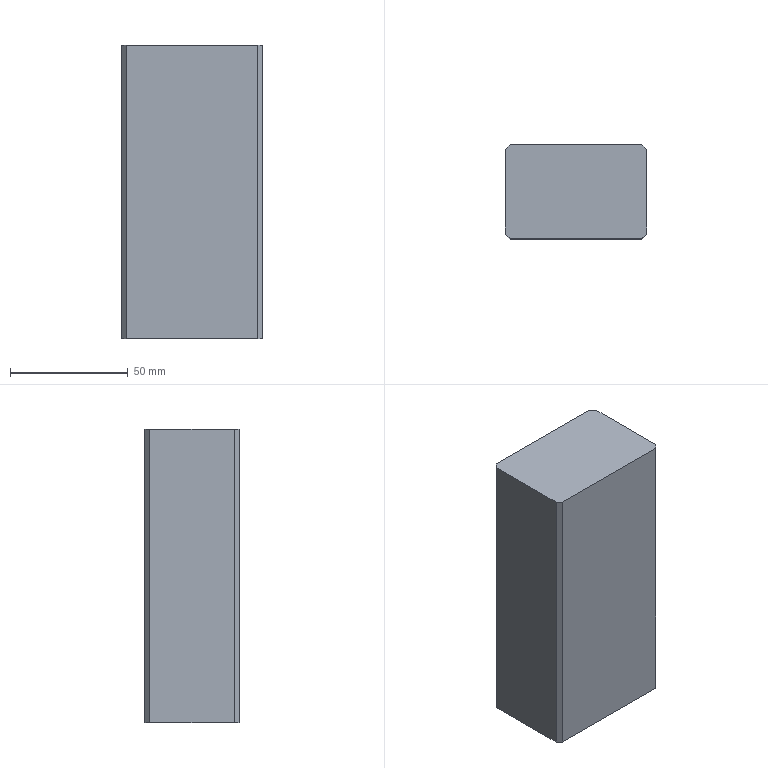Part | NX | features solid 2 | 1 solid | 10 faces | box 60 x 40 x 125 mm | volume 299000 mm3 | plane 10
STEP:
#1=CARTESIAN_POINT('',(428.,-270.,405.));
#2=VERTEX_POINT('',#1);
#3=CARTESIAN_POINT('',(372.,-270.,405.));
#4=VERTEX_POINT('',#3);
#5=CARTESIAN_POINT('',(430.,-270.,405.));
#6=DIRECTION('',(-1.,0.,0.));
#7=VECTOR('',#6,1000.);
#8=LINE('',#5,#7);
#9=EDGE_CURVE('',#2,#4,#8,.T.);
#10=ORIENTED_EDGE('',*,*,#9,.T.);
#11=CARTESIAN_POINT('',(370.,-272.,405.));
#12=VERTEX_POINT('',#11);
#13=CARTESIAN_POINT('',(401.,-241.,405.));
#14=DIRECTION('',(-0.7071,-0.7071,0.));
#15=VECTOR('',#14,1000.);
#16=LINE('',#13,#15);
#17=EDGE_CURVE('',#4,#12,#16,.T.);
#18=ORIENTED_EDGE('',*,*,#17,.T.);
#19=CARTESIAN_POINT('',(370.,-308.,405.));
#20=VERTEX_POINT('',#19);
#21=CARTESIAN_POINT('',(370.,-270.,405.));
#22=DIRECTION('',(0.,-1.,0.));
#23=VECTOR('',#22,1000.);
#24=LINE('',#21,#23);
#25=EDGE_CURVE('',#12,#20,#24,.T.);
#26=ORIENTED_EDGE('',*,*,#25,.T.);
#27=CARTESIAN_POINT('',(372.,-310.,405.));
#28=VERTEX_POINT('',#27);
#29=CARTESIAN_POINT('',(381.,-319.,405.));
#30=DIRECTION('',(-0.7071,0.7071,0.));
#31=VECTOR('',#30,1000.);
#32=LINE('',#29,#31);
#33=EDGE_CURVE('',#20,#28,#32,.F.);
#34=ORIENTED_EDGE('',*,*,#33,.T.);
#35=CARTESIAN_POINT('',(428.,-310.,405.));
#36=VERTEX_POINT('',#35);
#37=CARTESIAN_POINT('',(430.,-310.,405.));
#38=DIRECTION('',(-1.,0.,0.));
#39=VECTOR('',#38,1000.);
#40=LINE('',#37,#39);
#41=EDGE_CURVE('',#36,#28,#40,.T.);
#42=ORIENTED_EDGE('',*,*,#41,.F.);
#43=CARTESIAN_POINT('',(430.,-308.,405.));
#44=VERTEX_POINT('',#43);
#45=CARTESIAN_POINT('',(449.,-289.,405.));
#46=DIRECTION('',(0.7071,0.7071,0.));
#47=VECTOR('',#46,1000.);
#48=LINE('',#45,#47);
#49=EDGE_CURVE('',#36,#44,#48,.T.);
#50=ORIENTED_EDGE('',*,*,#49,.T.);
#51=CARTESIAN_POINT('',(430.,-272.,405.));
#52=VERTEX_POINT('',#51);
#53=CARTESIAN_POINT('',(430.,-270.,405.));
#54=DIRECTION('',(0.,1.,0.));
#55=VECTOR('',#54,1000.);
#56=LINE('',#53,#55);
#57=EDGE_CURVE('',#52,#44,#56,.F.);
#58=ORIENTED_EDGE('',*,*,#57,.F.);
#59=CARTESIAN_POINT('',(429.,-271.,405.));
#60=DIRECTION('',(0.7071,-0.7071,0.));
#61=VECTOR('',#60,1000.);
#62=LINE('',#59,#61);
#63=EDGE_CURVE('',#52,#2,#62,.F.);
#64=ORIENTED_EDGE('',*,*,#63,.T.);
#65=EDGE_LOOP('',(#10,#18,#26,#34,#42,#50,#58,#64));
#66=FACE_BOUND('',#65,.T.);
#67=CARTESIAN_POINT('',(430.,-270.,405.));
#68=DIRECTION('',(0.,0.,1.));
#69=DIRECTION('',(-1.,0.,0.));
#70=AXIS2_PLACEMENT_3D('',#67,#68,#69);
#71=PLANE('',#70);
#72=ADVANCED_FACE('',(#66),#71,.T.);
#73=ORIENTED_EDGE('',*,*,#25,.F.);
#74=CARTESIAN_POINT('',(370.,-272.,280.));
#75=VERTEX_POINT('',#74);
#76=CARTESIAN_POINT('',(370.,-272.,280.));
#77=DIRECTION('',(0.,0.,-1.));
#78=VECTOR('',#77,1000.);
#79=LINE('',#76,#78);
#80=EDGE_CURVE('',#12,#75,#79,.T.);
#81=ORIENTED_EDGE('',*,*,#80,.T.);
#82=CARTESIAN_POINT('',(370.,-308.,280.));
#83=VERTEX_POINT('',#82);
#84=CARTESIAN_POINT('',(370.,-270.,280.));
#85=DIRECTION('',(0.,1.,0.));
#86=VECTOR('',#85,1000.);
#87=LINE('',#84,#86);
#88=EDGE_CURVE('',#75,#83,#87,.F.);
#89=ORIENTED_EDGE('',*,*,#88,.T.);
#90=CARTESIAN_POINT('',(370.,-308.,420.));
#91=DIRECTION('',(0.,0.,1.));
#92=VECTOR('',#91,1000.);
#93=LINE('',#90,#92);
#94=EDGE_CURVE('',#83,#20,#93,.T.);
#95=ORIENTED_EDGE('',*,*,#94,.T.);
#96=EDGE_LOOP('',(#73,#81,#89,#95));
#97=FACE_BOUND('',#96,.T.);
#98=CARTESIAN_POINT('',(370.,-270.,420.));
#99=DIRECTION('',(-1.,0.,0.));
#100=DIRECTION('',(0.,0.,-1.));
#101=AXIS2_PLACEMENT_3D('',#98,#99,#100);
#102=PLANE('',#101);
#103=ADVANCED_FACE('',(#97),#102,.T.);
#104=ORIENTED_EDGE('',*,*,#88,.F.);
#105=CARTESIAN_POINT('',(372.,-270.,280.));
#106=VERTEX_POINT('',#105);
#107=CARTESIAN_POINT('',(401.,-241.,280.));
#108=DIRECTION('',(-0.7071,-0.7071,0.));
#109=VECTOR('',#108,1000.);
#110=LINE('',#107,#109);
#111=EDGE_CURVE('',#75,#106,#110,.F.);
#112=ORIENTED_EDGE('',*,*,#111,.T.);
#113=CARTESIAN_POINT('',(428.,-270.,280.));
#114=VERTEX_POINT('',#113);
#115=CARTESIAN_POINT('',(430.,-270.,280.));
#116=DIRECTION('',(1.,0.,0.));
#117=VECTOR('',#116,1000.);
#118=LINE('',#115,#117);
#119=EDGE_CURVE('',#114,#106,#118,.F.);
#120=ORIENTED_EDGE('',*,*,#119,.F.);
#121=CARTESIAN_POINT('',(430.,-272.,280.));
#122=VERTEX_POINT('',#121);
#123=CARTESIAN_POINT('',(429.,-271.,280.));
#124=DIRECTION('',(0.7071,-0.7071,0.));
#125=VECTOR('',#124,1000.);
#126=LINE('',#123,#125);
#127=EDGE_CURVE('',#114,#122,#126,.T.);
#128=ORIENTED_EDGE('',*,*,#127,.T.);
#129=CARTESIAN_POINT('',(430.,-308.,280.));
#130=VERTEX_POINT('',#129);
#131=CARTESIAN_POINT('',(430.,-270.,280.));
#132=DIRECTION('',(0.,-1.,0.));
#133=VECTOR('',#132,1000.);
#134=LINE('',#131,#133);
#135=EDGE_CURVE('',#122,#130,#134,.T.);
#136=ORIENTED_EDGE('',*,*,#135,.T.);
#137=CARTESIAN_POINT('',(428.,-310.,280.));
#138=VERTEX_POINT('',#137);
#139=CARTESIAN_POINT('',(449.,-289.,280.));
#140=DIRECTION('',(0.7071,0.7071,0.));
#141=VECTOR('',#140,1000.);
#142=LINE('',#139,#141);
#143=EDGE_CURVE('',#130,#138,#142,.F.);
#144=ORIENTED_EDGE('',*,*,#143,.T.);
#145=CARTESIAN_POINT('',(372.,-310.,280.));
#146=VERTEX_POINT('',#145);
#147=CARTESIAN_POINT('',(430.,-310.,280.));
#148=DIRECTION('',(1.,0.,0.));
#149=VECTOR('',#148,1000.);
#150=LINE('',#147,#149);
#151=EDGE_CURVE('',#138,#146,#150,.F.);
#152=ORIENTED_EDGE('',*,*,#151,.T.);
#153=CARTESIAN_POINT('',(381.,-319.,280.));
#154=DIRECTION('',(-0.7071,0.7071,0.));
#155=VECTOR('',#154,1000.);
#156=LINE('',#153,#155);
#157=EDGE_CURVE('',#146,#83,#156,.T.);
#158=ORIENTED_EDGE('',*,*,#157,.T.);
#159=EDGE_LOOP('',(#104,#112,#120,#128,#136,#144,#152,#158));
#160=FACE_BOUND('',#159,.T.);
#161=CARTESIAN_POINT('',(430.,-270.,280.));
#162=DIRECTION('',(0.,0.,1.));
#163=DIRECTION('',(-1.,0.,0.));
#164=AXIS2_PLACEMENT_3D('',#161,#162,#163);
#165=PLANE('',#164);
#166=ADVANCED_FACE('',(#160),#165,.F.);
#167=ORIENTED_EDGE('',*,*,#41,.T.);
#168=CARTESIAN_POINT('',(372.,-310.,420.));
#169=DIRECTION('',(0.,0.,-1.));
#170=VECTOR('',#169,1000.);
#171=LINE('',#168,#170);
#172=EDGE_CURVE('',#28,#146,#171,.T.);
#173=ORIENTED_EDGE('',*,*,#172,.T.);
#174=ORIENTED_EDGE('',*,*,#151,.F.);
#175=CARTESIAN_POINT('',(428.,-310.,420.));
#176=DIRECTION('',(0.,0.,1.));
#177=VECTOR('',#176,1000.);
#178=LINE('',#175,#177);
#179=EDGE_CURVE('',#138,#36,#178,.T.);
#180=ORIENTED_EDGE('',*,*,#179,.T.);
#181=EDGE_LOOP('',(#167,#173,#174,#180));
#182=FACE_BOUND('',#181,.T.);
#183=CARTESIAN_POINT('',(430.,-310.,420.));
#184=DIRECTION('',(0.,-1.,0.));
#185=DIRECTION('',(0.,0.,1.));
#186=AXIS2_PLACEMENT_3D('',#183,#184,#185);
#187=PLANE('',#186);
#188=ADVANCED_FACE('',(#182),#187,.T.);
#189=ORIENTED_EDGE('',*,*,#135,.F.);
#190=CARTESIAN_POINT('',(430.,-272.,405.));
#191=DIRECTION('',(0.,0.,-1.));
#192=VECTOR('',#191,1000.);
#193=LINE('',#190,#192);
#194=EDGE_CURVE('',#122,#52,#193,.F.);
#195=ORIENTED_EDGE('',*,*,#194,.T.);
#196=ORIENTED_EDGE('',*,*,#57,.T.);
#197=CARTESIAN_POINT('',(430.,-308.,420.));
#198=DIRECTION('',(0.,0.,1.));
#199=VECTOR('',#198,1000.);
#200=LINE('',#197,#199);
#201=EDGE_CURVE('',#44,#130,#200,.F.);
#202=ORIENTED_EDGE('',*,*,#201,.T.);
#203=EDGE_LOOP('',(#189,#195,#196,#202));
#204=FACE_BOUND('',#203,.T.);
#205=CARTESIAN_POINT('',(430.,-270.,420.));
#206=DIRECTION('',(-1.,0.,0.));
#207=DIRECTION('',(0.,0.,-1.));
#208=AXIS2_PLACEMENT_3D('',#205,#206,#207);
#209=PLANE('',#208);
#210=ADVANCED_FACE('',(#204),#209,.F.);
#211=ORIENTED_EDGE('',*,*,#119,.T.);
#212=CARTESIAN_POINT('',(372.,-270.,405.));
#213=DIRECTION('',(0.,0.,1.));
#214=VECTOR('',#213,1000.);
#215=LINE('',#212,#214);
#216=EDGE_CURVE('',#106,#4,#215,.T.);
#217=ORIENTED_EDGE('',*,*,#216,.T.);
#218=ORIENTED_EDGE('',*,*,#9,.F.);
#219=CARTESIAN_POINT('',(428.,-270.,280.));
#220=DIRECTION('',(0.,0.,-1.));
#221=VECTOR('',#220,1000.);
#222=LINE('',#219,#221);
#223=EDGE_CURVE('',#2,#114,#222,.T.);
#224=ORIENTED_EDGE('',*,*,#223,.T.);
#225=EDGE_LOOP('',(#211,#217,#218,#224));
#226=FACE_BOUND('',#225,.T.);
#227=CARTESIAN_POINT('',(430.,-270.,420.));
#228=DIRECTION('',(0.,-1.,0.));
#229=DIRECTION('',(0.,0.,1.));
#230=AXIS2_PLACEMENT_3D('',#227,#228,#229);
#231=PLANE('',#230);
#232=ADVANCED_FACE('',(#226),#231,.F.);
#233=ORIENTED_EDGE('',*,*,#17,.F.);
#234=ORIENTED_EDGE('',*,*,#216,.F.);
#235=ORIENTED_EDGE('',*,*,#111,.F.);
#236=ORIENTED_EDGE('',*,*,#80,.F.);
#237=EDGE_LOOP('',(#233,#234,#235,#236));
#238=FACE_BOUND('',#237,.T.);
#239=CARTESIAN_POINT('',(370.,-272.,420.));
#240=DIRECTION('',(-0.7071,0.7071,0.));
#241=DIRECTION('',(-0.7071,-0.7071,0.));
#242=AXIS2_PLACEMENT_3D('',#239,#240,#241);
#243=PLANE('',#242);
#244=ADVANCED_FACE('',(#238),#243,.T.);
#245=ORIENTED_EDGE('',*,*,#63,.F.);
#246=ORIENTED_EDGE('',*,*,#194,.F.);
#247=ORIENTED_EDGE('',*,*,#127,.F.);
#248=ORIENTED_EDGE('',*,*,#223,.F.);
#249=EDGE_LOOP('',(#245,#246,#247,#248));
#250=FACE_BOUND('',#249,.T.);
#251=CARTESIAN_POINT('',(428.,-270.,420.));
#252=DIRECTION('',(-0.7071,-0.7071,0.));
#253=DIRECTION('',(0.7071,-0.7071,0.));
#254=AXIS2_PLACEMENT_3D('',#251,#252,#253);
#255=PLANE('',#254);
#256=ADVANCED_FACE('',(#250),#255,.F.);
#257=ORIENTED_EDGE('',*,*,#33,.F.);
#258=ORIENTED_EDGE('',*,*,#94,.F.);
#259=ORIENTED_EDGE('',*,*,#157,.F.);
#260=ORIENTED_EDGE('',*,*,#172,.F.);
#261=EDGE_LOOP('',(#257,#258,#259,#260));
#262=FACE_BOUND('',#261,.T.);
#263=CARTESIAN_POINT('',(372.,-310.,420.));
#264=DIRECTION('',(0.7071,0.7071,0.));
#265=DIRECTION('',(-0.7071,0.7071,0.));
#266=AXIS2_PLACEMENT_3D('',#263,#264,#265);
#267=PLANE('',#266);
#268=ADVANCED_FACE('',(#262),#267,.F.);
#269=ORIENTED_EDGE('',*,*,#49,.F.);
#270=ORIENTED_EDGE('',*,*,#179,.F.);
#271=ORIENTED_EDGE('',*,*,#143,.F.);
#272=ORIENTED_EDGE('',*,*,#201,.F.);
#273=EDGE_LOOP('',(#269,#270,#271,#272));
#274=FACE_BOUND('',#273,.T.);
#275=CARTESIAN_POINT('',(430.,-308.,420.));
#276=DIRECTION('',(0.7071,-0.7071,0.));
#277=DIRECTION('',(0.7071,0.7071,0.));
#278=AXIS2_PLACEMENT_3D('',#275,#276,#277);
#279=PLANE('',#278);
#280=ADVANCED_FACE('',(#274),#279,.T.);
#281=CLOSED_SHELL('',(#72,#103,#166,#188,#210,#232,#244,#256,#268,#280));
#282=MANIFOLD_SOLID_BREP('',#281);
#283=(LENGTH_UNIT()NAMED_UNIT(*)SI_UNIT(.MILLI.,.METRE.));
#284=UNCERTAINTY_MEASURE_WITH_UNIT(LENGTH_MEASURE(0.00001),#283,'','');
#285=(NAMED_UNIT(*)PLANE_ANGLE_UNIT()SI_UNIT($,.RADIAN.));
#286=(NAMED_UNIT(*)SI_UNIT($,.STERADIAN.)SOLID_ANGLE_UNIT());
#287=(GEOMETRIC_REPRESENTATION_CONTEXT(3)GLOBAL_UNCERTAINTY_ASSIGNED_CONTEXT((#284))GLOBAL_UNIT_ASSIGNED_CONTEXT((#283,#285,#286))REPRESENTATION_CONTEXT('',''));
#288=ADVANCED_BREP_SHAPE_REPRESENTATION('',(#282),#287);